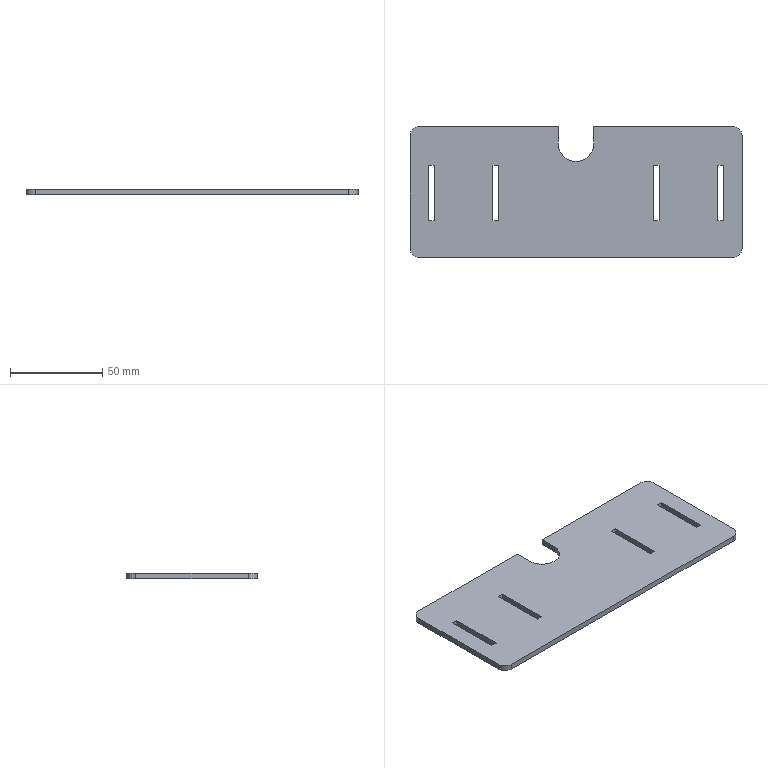Part | SolidWorks | features FlatPattern 1, SMBaseFlange 1, SheetMetal 1 | 1 solid | 30 faces | box 180 x 71 x 3.2 mm | volume 38567 mm3 | plane 25 | cylinder 5 | commonest cylinder face diameters 10 x4 19 x1
STEP:
#1=CARTESIAN_POINT('',(43.2,-230.5,3.2));
#2=VERTEX_POINT('',#1);
#3=CARTESIAN_POINT('',(48.2,-225.5,3.2));
#4=VERTEX_POINT('',#3);
#5=CARTESIAN_POINT('',(43.2,-225.5,3.2));
#6=DIRECTION('',(0.,0.,1.));
#7=DIRECTION('',(1.,0.,0.));
#8=AXIS2_PLACEMENT_3D('',#5,#6,#7);
#9=CIRCLE('',#8,5.);
#10=EDGE_CURVE('',#2,#4,#9,.T.);
#11=ORIENTED_EDGE('',*,*,#10,.T.);
#12=CARTESIAN_POINT('',(48.2,-164.5,3.2));
#13=VERTEX_POINT('',#12);
#14=CARTESIAN_POINT('',(48.2,-164.5,3.2));
#15=DIRECTION('',(0.,1.,0.));
#16=VECTOR('',#15,1000.);
#17=LINE('',#14,#16);
#18=EDGE_CURVE('',#4,#13,#17,.T.);
#19=ORIENTED_EDGE('',*,*,#18,.T.);
#20=CARTESIAN_POINT('',(43.2,-159.5,3.2));
#21=VERTEX_POINT('',#20);
#22=CARTESIAN_POINT('',(43.2,-164.5,3.2));
#23=DIRECTION('',(0.,0.,1.));
#24=DIRECTION('',(1.,0.,0.));
#25=AXIS2_PLACEMENT_3D('',#22,#23,#24);
#26=CIRCLE('',#25,5.);
#27=EDGE_CURVE('',#13,#21,#26,.T.);
#28=ORIENTED_EDGE('',*,*,#27,.T.);
#29=CARTESIAN_POINT('',(-32.3,-159.5,3.2));
#30=VERTEX_POINT('',#29);
#31=CARTESIAN_POINT('',(43.2,-159.5,3.2));
#32=DIRECTION('',(-1.,0.,0.));
#33=VECTOR('',#32,1000.);
#34=LINE('',#31,#33);
#35=EDGE_CURVE('',#21,#30,#34,.T.);
#36=ORIENTED_EDGE('',*,*,#35,.T.);
#37=CARTESIAN_POINT('',(-32.3,-169.,3.2));
#38=VERTEX_POINT('',#37);
#39=CARTESIAN_POINT('',(-32.3,-169.,3.2));
#40=DIRECTION('',(0.,-1.,0.));
#41=VECTOR('',#40,1000.);
#42=LINE('',#39,#41);
#43=EDGE_CURVE('',#30,#38,#42,.T.);
#44=ORIENTED_EDGE('',*,*,#43,.T.);
#45=CARTESIAN_POINT('',(-51.3,-169.,3.2));
#46=VERTEX_POINT('',#45);
#47=CARTESIAN_POINT('',(-41.8,-169.,3.2));
#48=DIRECTION('',(0.,0.,-1.));
#49=DIRECTION('',(1.,0.,0.));
#50=AXIS2_PLACEMENT_3D('',#47,#48,#49);
#51=CIRCLE('',#50,9.5);
#52=EDGE_CURVE('',#38,#46,#51,.T.);
#53=ORIENTED_EDGE('',*,*,#52,.T.);
#54=CARTESIAN_POINT('',(-51.3,-159.5,3.2));
#55=VERTEX_POINT('',#54);
#56=CARTESIAN_POINT('',(-51.3,-169.,3.2));
#57=DIRECTION('',(0.,1.,0.));
#58=VECTOR('',#57,1000.);
#59=LINE('',#56,#58);
#60=EDGE_CURVE('',#46,#55,#59,.T.);
#61=ORIENTED_EDGE('',*,*,#60,.T.);
#62=CARTESIAN_POINT('',(-126.8,-159.5,3.2));
#63=VERTEX_POINT('',#62);
#64=CARTESIAN_POINT('',(-51.3,-159.5,3.2));
#65=DIRECTION('',(-1.,0.,0.));
#66=VECTOR('',#65,1000.);
#67=LINE('',#64,#66);
#68=EDGE_CURVE('',#55,#63,#67,.T.);
#69=ORIENTED_EDGE('',*,*,#68,.T.);
#70=CARTESIAN_POINT('',(-131.8,-164.5,3.2));
#71=VERTEX_POINT('',#70);
#72=CARTESIAN_POINT('',(-126.8,-164.5,3.2));
#73=DIRECTION('',(0.,0.,1.));
#74=DIRECTION('',(-1.,0.,0.));
#75=AXIS2_PLACEMENT_3D('',#72,#73,#74);
#76=CIRCLE('',#75,5.);
#77=EDGE_CURVE('',#63,#71,#76,.T.);
#78=ORIENTED_EDGE('',*,*,#77,.T.);
#79=CARTESIAN_POINT('',(-131.8,-225.5,3.2));
#80=VERTEX_POINT('',#79);
#81=CARTESIAN_POINT('',(-131.8,-164.5,3.2));
#82=DIRECTION('',(0.,-1.,0.));
#83=VECTOR('',#82,1000.);
#84=LINE('',#81,#83);
#85=EDGE_CURVE('',#71,#80,#84,.T.);
#86=ORIENTED_EDGE('',*,*,#85,.T.);
#87=CARTESIAN_POINT('',(-126.8,-230.5,3.2));
#88=VERTEX_POINT('',#87);
#89=CARTESIAN_POINT('',(-126.8,-225.5,3.2));
#90=DIRECTION('',(0.,0.,1.));
#91=DIRECTION('',(-1.,0.,0.));
#92=AXIS2_PLACEMENT_3D('',#89,#90,#91);
#93=CIRCLE('',#92,5.);
#94=EDGE_CURVE('',#80,#88,#93,.T.);
#95=ORIENTED_EDGE('',*,*,#94,.T.);
#96=CARTESIAN_POINT('',(43.2,-230.5,3.2));
#97=DIRECTION('',(1.,0.,0.));
#98=VECTOR('',#97,1000.);
#99=LINE('',#96,#98);
#100=EDGE_CURVE('',#88,#2,#99,.T.);
#101=ORIENTED_EDGE('',*,*,#100,.T.);
#102=EDGE_LOOP('',(#11,#19,#28,#36,#44,#53,#61,#69,#78,#86,#95,#101));
#103=FACE_OUTER_BOUND('',#102,.T.);
#104=CARTESIAN_POINT('',(-121.8,-210.5,3.2));
#105=VERTEX_POINT('',#104);
#106=CARTESIAN_POINT('',(-118.6,-210.5,3.2));
#107=VERTEX_POINT('',#106);
#108=CARTESIAN_POINT('',(-121.8,-210.5,3.2));
#109=DIRECTION('',(1.,0.,0.));
#110=VECTOR('',#109,1000.);
#111=LINE('',#108,#110);
#112=EDGE_CURVE('',#105,#107,#111,.T.);
#113=ORIENTED_EDGE('',*,*,#112,.F.);
#114=CARTESIAN_POINT('',(-121.8,-180.5,3.2));
#115=VERTEX_POINT('',#114);
#116=CARTESIAN_POINT('',(-121.8,-210.5,3.2));
#117=DIRECTION('',(0.,-1.,0.));
#118=VECTOR('',#117,1000.);
#119=LINE('',#116,#118);
#120=EDGE_CURVE('',#115,#105,#119,.T.);
#121=ORIENTED_EDGE('',*,*,#120,.F.);
#122=CARTESIAN_POINT('',(-118.6,-180.5,3.2));
#123=VERTEX_POINT('',#122);
#124=CARTESIAN_POINT('',(-121.8,-180.5,3.2));
#125=DIRECTION('',(-1.,0.,0.));
#126=VECTOR('',#125,1000.);
#127=LINE('',#124,#126);
#128=EDGE_CURVE('',#123,#115,#127,.T.);
#129=ORIENTED_EDGE('',*,*,#128,.F.);
#130=CARTESIAN_POINT('',(-118.6,-210.5,3.2));
#131=DIRECTION('',(0.,1.,0.));
#132=VECTOR('',#131,1000.);
#133=LINE('',#130,#132);
#134=EDGE_CURVE('',#107,#123,#133,.T.);
#135=ORIENTED_EDGE('',*,*,#134,.F.);
#136=EDGE_LOOP('',(#113,#121,#129,#135));
#137=FACE_BOUND('',#136,.T.);
#138=CARTESIAN_POINT('',(-86.8,-210.5,3.2));
#139=VERTEX_POINT('',#138);
#140=CARTESIAN_POINT('',(-83.6,-210.5,3.2));
#141=VERTEX_POINT('',#140);
#142=CARTESIAN_POINT('',(-86.8,-210.5,3.2));
#143=DIRECTION('',(1.,0.,0.));
#144=VECTOR('',#143,1000.);
#145=LINE('',#142,#144);
#146=EDGE_CURVE('',#139,#141,#145,.T.);
#147=ORIENTED_EDGE('',*,*,#146,.F.);
#148=CARTESIAN_POINT('',(-86.8,-180.5,3.2));
#149=VERTEX_POINT('',#148);
#150=CARTESIAN_POINT('',(-86.8,-210.5,3.2));
#151=DIRECTION('',(0.,-1.,0.));
#152=VECTOR('',#151,1000.);
#153=LINE('',#150,#152);
#154=EDGE_CURVE('',#149,#139,#153,.T.);
#155=ORIENTED_EDGE('',*,*,#154,.F.);
#156=CARTESIAN_POINT('',(-83.6,-180.5,3.2));
#157=VERTEX_POINT('',#156);
#158=CARTESIAN_POINT('',(-86.8,-180.5,3.2));
#159=DIRECTION('',(-1.,0.,0.));
#160=VECTOR('',#159,1000.);
#161=LINE('',#158,#160);
#162=EDGE_CURVE('',#157,#149,#161,.T.);
#163=ORIENTED_EDGE('',*,*,#162,.F.);
#164=CARTESIAN_POINT('',(-83.6,-210.5,3.2));
#165=DIRECTION('',(0.,1.,0.));
#166=VECTOR('',#165,1000.);
#167=LINE('',#164,#166);
#168=EDGE_CURVE('',#141,#157,#167,.T.);
#169=ORIENTED_EDGE('',*,*,#168,.F.);
#170=EDGE_LOOP('',(#147,#155,#163,#169));
#171=FACE_BOUND('',#170,.T.);
#172=CARTESIAN_POINT('',(0.,-210.5,3.2));
#173=VERTEX_POINT('',#172);
#174=CARTESIAN_POINT('',(3.2,-210.5,3.2));
#175=VERTEX_POINT('',#174);
#176=CARTESIAN_POINT('',(0.,-210.5,3.2));
#177=DIRECTION('',(1.,0.,0.));
#178=VECTOR('',#177,1000.);
#179=LINE('',#176,#178);
#180=EDGE_CURVE('',#173,#175,#179,.T.);
#181=ORIENTED_EDGE('',*,*,#180,.F.);
#182=CARTESIAN_POINT('',(0.,-180.5,3.2));
#183=VERTEX_POINT('',#182);
#184=CARTESIAN_POINT('',(0.,-210.5,3.2));
#185=DIRECTION('',(0.,-1.,0.));
#186=VECTOR('',#185,1000.);
#187=LINE('',#184,#186);
#188=EDGE_CURVE('',#183,#173,#187,.T.);
#189=ORIENTED_EDGE('',*,*,#188,.F.);
#190=CARTESIAN_POINT('',(3.2,-180.5,3.2));
#191=VERTEX_POINT('',#190);
#192=CARTESIAN_POINT('',(0.,-180.5,3.2));
#193=DIRECTION('',(-1.,0.,0.));
#194=VECTOR('',#193,1000.);
#195=LINE('',#192,#194);
#196=EDGE_CURVE('',#191,#183,#195,.T.);
#197=ORIENTED_EDGE('',*,*,#196,.F.);
#198=CARTESIAN_POINT('',(3.2,-210.5,3.2));
#199=DIRECTION('',(0.,1.,0.));
#200=VECTOR('',#199,1000.);
#201=LINE('',#198,#200);
#202=EDGE_CURVE('',#175,#191,#201,.T.);
#203=ORIENTED_EDGE('',*,*,#202,.F.);
#204=EDGE_LOOP('',(#181,#189,#197,#203));
#205=FACE_BOUND('',#204,.T.);
#206=CARTESIAN_POINT('',(35.,-210.5,3.2));
#207=VERTEX_POINT('',#206);
#208=CARTESIAN_POINT('',(38.2,-210.5,3.2));
#209=VERTEX_POINT('',#208);
#210=CARTESIAN_POINT('',(35.,-210.5,3.2));
#211=DIRECTION('',(1.,0.,0.));
#212=VECTOR('',#211,1000.);
#213=LINE('',#210,#212);
#214=EDGE_CURVE('',#207,#209,#213,.T.);
#215=ORIENTED_EDGE('',*,*,#214,.F.);
#216=CARTESIAN_POINT('',(35.,-180.5,3.2));
#217=VERTEX_POINT('',#216);
#218=CARTESIAN_POINT('',(35.,-210.5,3.2));
#219=DIRECTION('',(0.,-1.,0.));
#220=VECTOR('',#219,1000.);
#221=LINE('',#218,#220);
#222=EDGE_CURVE('',#217,#207,#221,.T.);
#223=ORIENTED_EDGE('',*,*,#222,.F.);
#224=CARTESIAN_POINT('',(38.2,-180.5,3.2));
#225=VERTEX_POINT('',#224);
#226=CARTESIAN_POINT('',(35.,-180.5,3.2));
#227=DIRECTION('',(-1.,0.,0.));
#228=VECTOR('',#227,1000.);
#229=LINE('',#226,#228);
#230=EDGE_CURVE('',#225,#217,#229,.T.);
#231=ORIENTED_EDGE('',*,*,#230,.F.);
#232=CARTESIAN_POINT('',(38.2,-210.5,3.2));
#233=DIRECTION('',(0.,1.,0.));
#234=VECTOR('',#233,1000.);
#235=LINE('',#232,#234);
#236=EDGE_CURVE('',#209,#225,#235,.T.);
#237=ORIENTED_EDGE('',*,*,#236,.F.);
#238=EDGE_LOOP('',(#215,#223,#231,#237));
#239=FACE_BOUND('',#238,.T.);
#240=CARTESIAN_POINT('',(43.2,-225.5,3.2));
#241=DIRECTION('',(0.,0.,1.));
#242=DIRECTION('',(1.,0.,0.));
#243=AXIS2_PLACEMENT_3D('',#240,#241,#242);
#244=PLANE('',#243);
#245=ADVANCED_FACE('',(#103,#137,#171,#205,#239),#244,.T.);
#246=CARTESIAN_POINT('',(0.,-180.5,0.));
#247=VERTEX_POINT('',#246);
#248=CARTESIAN_POINT('',(0.,-210.5,0.));
#249=VERTEX_POINT('',#248);
#250=CARTESIAN_POINT('',(0.,-210.5,0.));
#251=DIRECTION('',(0.,-1.,0.));
#252=VECTOR('',#251,1000.);
#253=LINE('',#250,#252);
#254=EDGE_CURVE('',#247,#249,#253,.T.);
#255=ORIENTED_EDGE('',*,*,#254,.T.);
#256=CARTESIAN_POINT('',(3.2,-210.5,0.));
#257=VERTEX_POINT('',#256);
#258=CARTESIAN_POINT('',(0.,-210.5,0.));
#259=DIRECTION('',(1.,0.,0.));
#260=VECTOR('',#259,1000.);
#261=LINE('',#258,#260);
#262=EDGE_CURVE('',#249,#257,#261,.T.);
#263=ORIENTED_EDGE('',*,*,#262,.T.);
#264=CARTESIAN_POINT('',(3.2,-180.5,0.));
#265=VERTEX_POINT('',#264);
#266=CARTESIAN_POINT('',(3.2,-210.5,0.));
#267=DIRECTION('',(0.,1.,0.));
#268=VECTOR('',#267,1000.);
#269=LINE('',#266,#268);
#270=EDGE_CURVE('',#257,#265,#269,.T.);
#271=ORIENTED_EDGE('',*,*,#270,.T.);
#272=CARTESIAN_POINT('',(0.,-180.5,0.));
#273=DIRECTION('',(-1.,0.,0.));
#274=VECTOR('',#273,1000.);
#275=LINE('',#272,#274);
#276=EDGE_CURVE('',#265,#247,#275,.T.);
#277=ORIENTED_EDGE('',*,*,#276,.T.);
#278=EDGE_LOOP('',(#255,#263,#271,#277));
#279=FACE_BOUND('',#278,.T.);
#280=CARTESIAN_POINT('',(-121.8,-180.5,0.));
#281=VERTEX_POINT('',#280);
#282=CARTESIAN_POINT('',(-121.8,-210.5,0.));
#283=VERTEX_POINT('',#282);
#284=CARTESIAN_POINT('',(-121.8,-210.5,0.));
#285=DIRECTION('',(0.,-1.,0.));
#286=VECTOR('',#285,1000.);
#287=LINE('',#284,#286);
#288=EDGE_CURVE('',#281,#283,#287,.T.);
#289=ORIENTED_EDGE('',*,*,#288,.T.);
#290=CARTESIAN_POINT('',(-118.6,-210.5,0.));
#291=VERTEX_POINT('',#290);
#292=CARTESIAN_POINT('',(-121.8,-210.5,0.));
#293=DIRECTION('',(1.,0.,0.));
#294=VECTOR('',#293,1000.);
#295=LINE('',#292,#294);
#296=EDGE_CURVE('',#283,#291,#295,.T.);
#297=ORIENTED_EDGE('',*,*,#296,.T.);
#298=CARTESIAN_POINT('',(-118.6,-180.5,0.));
#299=VERTEX_POINT('',#298);
#300=CARTESIAN_POINT('',(-118.6,-210.5,0.));
#301=DIRECTION('',(0.,1.,0.));
#302=VECTOR('',#301,1000.);
#303=LINE('',#300,#302);
#304=EDGE_CURVE('',#291,#299,#303,.T.);
#305=ORIENTED_EDGE('',*,*,#304,.T.);
#306=CARTESIAN_POINT('',(-121.8,-180.5,0.));
#307=DIRECTION('',(-1.,0.,0.));
#308=VECTOR('',#307,1000.);
#309=LINE('',#306,#308);
#310=EDGE_CURVE('',#299,#281,#309,.T.);
#311=ORIENTED_EDGE('',*,*,#310,.T.);
#312=EDGE_LOOP('',(#289,#297,#305,#311));
#313=FACE_BOUND('',#312,.T.);
#314=CARTESIAN_POINT('',(43.2,-230.5,0.));
#315=VERTEX_POINT('',#314);
#316=CARTESIAN_POINT('',(48.2,-225.5,0.));
#317=VERTEX_POINT('',#316);
#318=CARTESIAN_POINT('',(43.2,-225.5,0.));
#319=DIRECTION('',(0.,0.,1.));
#320=DIRECTION('',(1.,0.,0.));
#321=AXIS2_PLACEMENT_3D('',#318,#319,#320);
#322=CIRCLE('',#321,5.);
#323=EDGE_CURVE('',#315,#317,#322,.T.);
#324=ORIENTED_EDGE('',*,*,#323,.F.);
#325=CARTESIAN_POINT('',(-126.8,-230.5,0.));
#326=VERTEX_POINT('',#325);
#327=CARTESIAN_POINT('',(43.2,-230.5,0.));
#328=DIRECTION('',(1.,0.,0.));
#329=VECTOR('',#328,1000.);
#330=LINE('',#327,#329);
#331=EDGE_CURVE('',#326,#315,#330,.T.);
#332=ORIENTED_EDGE('',*,*,#331,.F.);
#333=CARTESIAN_POINT('',(-131.8,-225.5,0.));
#334=VERTEX_POINT('',#333);
#335=CARTESIAN_POINT('',(-126.8,-225.5,0.));
#336=DIRECTION('',(0.,0.,1.));
#337=DIRECTION('',(-1.,0.,0.));
#338=AXIS2_PLACEMENT_3D('',#335,#336,#337);
#339=CIRCLE('',#338,5.);
#340=EDGE_CURVE('',#334,#326,#339,.T.);
#341=ORIENTED_EDGE('',*,*,#340,.F.);
#342=CARTESIAN_POINT('',(-131.8,-164.5,0.));
#343=VERTEX_POINT('',#342);
#344=CARTESIAN_POINT('',(-131.8,-164.5,0.));
#345=DIRECTION('',(0.,-1.,0.));
#346=VECTOR('',#345,1000.);
#347=LINE('',#344,#346);
#348=EDGE_CURVE('',#343,#334,#347,.T.);
#349=ORIENTED_EDGE('',*,*,#348,.F.);
#350=CARTESIAN_POINT('',(-126.8,-159.5,0.));
#351=VERTEX_POINT('',#350);
#352=CARTESIAN_POINT('',(-126.8,-164.5,0.));
#353=DIRECTION('',(0.,0.,1.));
#354=DIRECTION('',(-1.,0.,0.));
#355=AXIS2_PLACEMENT_3D('',#352,#353,#354);
#356=CIRCLE('',#355,5.);
#357=EDGE_CURVE('',#351,#343,#356,.T.);
#358=ORIENTED_EDGE('',*,*,#357,.F.);
#359=CARTESIAN_POINT('',(-51.3,-159.5,0.));
#360=VERTEX_POINT('',#359);
#361=CARTESIAN_POINT('',(-51.3,-159.5,0.));
#362=DIRECTION('',(-1.,0.,0.));
#363=VECTOR('',#362,1000.);
#364=LINE('',#361,#363);
#365=EDGE_CURVE('',#360,#351,#364,.T.);
#366=ORIENTED_EDGE('',*,*,#365,.F.);
#367=CARTESIAN_POINT('',(-51.3,-169.,0.));
#368=VERTEX_POINT('',#367);
#369=CARTESIAN_POINT('',(-51.3,-169.,0.));
#370=DIRECTION('',(0.,1.,0.));
#371=VECTOR('',#370,1000.);
#372=LINE('',#369,#371);
#373=EDGE_CURVE('',#368,#360,#372,.T.);
#374=ORIENTED_EDGE('',*,*,#373,.F.);
#375=CARTESIAN_POINT('',(-32.3,-169.,0.));
#376=VERTEX_POINT('',#375);
#377=CARTESIAN_POINT('',(-41.8,-169.,0.));
#378=DIRECTION('',(0.,0.,-1.));
#379=DIRECTION('',(1.,0.,0.));
#380=AXIS2_PLACEMENT_3D('',#377,#378,#379);
#381=CIRCLE('',#380,9.5);
#382=EDGE_CURVE('',#376,#368,#381,.T.);
#383=ORIENTED_EDGE('',*,*,#382,.F.);
#384=CARTESIAN_POINT('',(-32.3,-159.5,0.));
#385=VERTEX_POINT('',#384);
#386=CARTESIAN_POINT('',(-32.3,-169.,0.));
#387=DIRECTION('',(0.,-1.,0.));
#388=VECTOR('',#387,1000.);
#389=LINE('',#386,#388);
#390=EDGE_CURVE('',#385,#376,#389,.T.);
#391=ORIENTED_EDGE('',*,*,#390,.F.);
#392=CARTESIAN_POINT('',(43.2,-159.5,0.));
#393=VERTEX_POINT('',#392);
#394=CARTESIAN_POINT('',(43.2,-159.5,0.));
#395=DIRECTION('',(-1.,0.,0.));
#396=VECTOR('',#395,1000.);
#397=LINE('',#394,#396);
#398=EDGE_CURVE('',#393,#385,#397,.T.);
#399=ORIENTED_EDGE('',*,*,#398,.F.);
#400=CARTESIAN_POINT('',(48.2,-164.5,0.));
#401=VERTEX_POINT('',#400);
#402=CARTESIAN_POINT('',(43.2,-164.5,0.));
#403=DIRECTION('',(0.,0.,1.));
#404=DIRECTION('',(1.,0.,0.));
#405=AXIS2_PLACEMENT_3D('',#402,#403,#404);
#406=CIRCLE('',#405,5.);
#407=EDGE_CURVE('',#401,#393,#406,.T.);
#408=ORIENTED_EDGE('',*,*,#407,.F.);
#409=CARTESIAN_POINT('',(48.2,-164.5,0.));
#410=DIRECTION('',(0.,1.,0.));
#411=VECTOR('',#410,1000.);
#412=LINE('',#409,#411);
#413=EDGE_CURVE('',#317,#401,#412,.T.);
#414=ORIENTED_EDGE('',*,*,#413,.F.);
#415=EDGE_LOOP('',(#324,#332,#341,#349,#358,#366,#374,#383,#391,#399,#408,#414));
#416=FACE_OUTER_BOUND('',#415,.T.);
#417=CARTESIAN_POINT('',(-86.8,-180.5,0.));
#418=VERTEX_POINT('',#417);
#419=CARTESIAN_POINT('',(-86.8,-210.5,0.));
#420=VERTEX_POINT('',#419);
#421=CARTESIAN_POINT('',(-86.8,-210.5,0.));
#422=DIRECTION('',(0.,-1.,0.));
#423=VECTOR('',#422,1000.);
#424=LINE('',#421,#423);
#425=EDGE_CURVE('',#418,#420,#424,.T.);
#426=ORIENTED_EDGE('',*,*,#425,.T.);
#427=CARTESIAN_POINT('',(-83.6,-210.5,0.));
#428=VERTEX_POINT('',#427);
#429=CARTESIAN_POINT('',(-86.8,-210.5,0.));
#430=DIRECTION('',(1.,0.,0.));
#431=VECTOR('',#430,1000.);
#432=LINE('',#429,#431);
#433=EDGE_CURVE('',#420,#428,#432,.T.);
#434=ORIENTED_EDGE('',*,*,#433,.T.);
#435=CARTESIAN_POINT('',(-83.6,-180.5,0.));
#436=VERTEX_POINT('',#435);
#437=CARTESIAN_POINT('',(-83.6,-210.5,0.));
#438=DIRECTION('',(0.,1.,0.));
#439=VECTOR('',#438,1000.);
#440=LINE('',#437,#439);
#441=EDGE_CURVE('',#428,#436,#440,.T.);
#442=ORIENTED_EDGE('',*,*,#441,.T.);
#443=CARTESIAN_POINT('',(-86.8,-180.5,0.));
#444=DIRECTION('',(-1.,0.,0.));
#445=VECTOR('',#444,1000.);
#446=LINE('',#443,#445);
#447=EDGE_CURVE('',#436,#418,#446,.T.);
#448=ORIENTED_EDGE('',*,*,#447,.T.);
#449=EDGE_LOOP('',(#426,#434,#442,#448));
#450=FACE_BOUND('',#449,.T.);
#451=CARTESIAN_POINT('',(35.,-180.5,0.));
#452=VERTEX_POINT('',#451);
#453=CARTESIAN_POINT('',(35.,-210.5,0.));
#454=VERTEX_POINT('',#453);
#455=CARTESIAN_POINT('',(35.,-210.5,0.));
#456=DIRECTION('',(0.,-1.,0.));
#457=VECTOR('',#456,1000.);
#458=LINE('',#455,#457);
#459=EDGE_CURVE('',#452,#454,#458,.T.);
#460=ORIENTED_EDGE('',*,*,#459,.T.);
#461=CARTESIAN_POINT('',(38.2,-210.5,0.));
#462=VERTEX_POINT('',#461);
#463=CARTESIAN_POINT('',(35.,-210.5,0.));
#464=DIRECTION('',(1.,0.,0.));
#465=VECTOR('',#464,1000.);
#466=LINE('',#463,#465);
#467=EDGE_CURVE('',#454,#462,#466,.T.);
#468=ORIENTED_EDGE('',*,*,#467,.T.);
#469=CARTESIAN_POINT('',(38.2,-180.5,0.));
#470=VERTEX_POINT('',#469);
#471=CARTESIAN_POINT('',(38.2,-210.5,0.));
#472=DIRECTION('',(0.,1.,0.));
#473=VECTOR('',#472,1000.);
#474=LINE('',#471,#473);
#475=EDGE_CURVE('',#462,#470,#474,.T.);
#476=ORIENTED_EDGE('',*,*,#475,.T.);
#477=CARTESIAN_POINT('',(35.,-180.5,0.));
#478=DIRECTION('',(-1.,0.,0.));
#479=VECTOR('',#478,1000.);
#480=LINE('',#477,#479);
#481=EDGE_CURVE('',#470,#452,#480,.T.);
#482=ORIENTED_EDGE('',*,*,#481,.T.);
#483=EDGE_LOOP('',(#460,#468,#476,#482));
#484=FACE_BOUND('',#483,.T.);
#485=CARTESIAN_POINT('',(43.2,-225.5,0.));
#486=DIRECTION('',(0.,0.,1.));
#487=DIRECTION('',(1.,0.,0.));
#488=AXIS2_PLACEMENT_3D('',#485,#486,#487);
#489=PLANE('',#488);
#490=ADVANCED_FACE('',(#279,#313,#416,#450,#484),#489,.F.);
#491=ORIENTED_EDGE('',*,*,#323,.T.);
#492=CARTESIAN_POINT('',(48.2,-225.5,3.2));
#493=DIRECTION('',(0.,0.,-1.));
#494=VECTOR('',#493,1000.);
#495=LINE('',#492,#494);
#496=EDGE_CURVE('',#4,#317,#495,.T.);
#497=ORIENTED_EDGE('',*,*,#496,.F.);
#498=ORIENTED_EDGE('',*,*,#10,.F.);
#499=CARTESIAN_POINT('',(43.2,-230.5,3.2));
#500=DIRECTION('',(0.,0.,-1.));
#501=VECTOR('',#500,1000.);
#502=LINE('',#499,#501);
#503=EDGE_CURVE('',#2,#315,#502,.T.);
#504=ORIENTED_EDGE('',*,*,#503,.T.);
#505=EDGE_LOOP('',(#491,#497,#498,#504));
#506=FACE_OUTER_BOUND('',#505,.T.);
#507=CARTESIAN_POINT('',(43.2,-225.5,3.2));
#508=DIRECTION('',(0.,0.,-1.));
#509=DIRECTION('',(-1.,0.,0.));
#510=AXIS2_PLACEMENT_3D('',#507,#508,#509);
#511=CYLINDRICAL_SURFACE('',#510,5.);
#512=ADVANCED_FACE('',(#506),#511,.T.);
#513=ORIENTED_EDGE('',*,*,#413,.T.);
#514=CARTESIAN_POINT('',(48.2,-164.5,3.2));
#515=DIRECTION('',(0.,0.,-1.));
#516=VECTOR('',#515,1000.);
#517=LINE('',#514,#516);
#518=EDGE_CURVE('',#13,#401,#517,.T.);
#519=ORIENTED_EDGE('',*,*,#518,.F.);
#520=ORIENTED_EDGE('',*,*,#18,.F.);
#521=ORIENTED_EDGE('',*,*,#496,.T.);
#522=EDGE_LOOP('',(#513,#519,#520,#521));
#523=FACE_OUTER_BOUND('',#522,.T.);
#524=CARTESIAN_POINT('',(48.2,-164.5,3.2));
#525=DIRECTION('',(-1.,0.,0.));
#526=DIRECTION('',(0.,-1.,0.));
#527=AXIS2_PLACEMENT_3D('',#524,#525,#526);
#528=PLANE('',#527);
#529=ADVANCED_FACE('',(#523),#528,.F.);
#530=ORIENTED_EDGE('',*,*,#407,.T.);
#531=CARTESIAN_POINT('',(43.2,-159.5,3.2));
#532=DIRECTION('',(0.,0.,-1.));
#533=VECTOR('',#532,1000.);
#534=LINE('',#531,#533);
#535=EDGE_CURVE('',#21,#393,#534,.T.);
#536=ORIENTED_EDGE('',*,*,#535,.F.);
#537=ORIENTED_EDGE('',*,*,#27,.F.);
#538=ORIENTED_EDGE('',*,*,#518,.T.);
#539=EDGE_LOOP('',(#530,#536,#537,#538));
#540=FACE_OUTER_BOUND('',#539,.T.);
#541=CARTESIAN_POINT('',(43.2,-164.5,3.2));
#542=DIRECTION('',(0.,0.,-1.));
#543=DIRECTION('',(-1.,0.,0.));
#544=AXIS2_PLACEMENT_3D('',#541,#542,#543);
#545=CYLINDRICAL_SURFACE('',#544,5.);
#546=ADVANCED_FACE('',(#540),#545,.T.);
#547=ORIENTED_EDGE('',*,*,#398,.T.);
#548=CARTESIAN_POINT('',(-32.3,-159.5,3.2));
#549=DIRECTION('',(0.,0.,-1.));
#550=VECTOR('',#549,1000.);
#551=LINE('',#548,#550);
#552=EDGE_CURVE('',#30,#385,#551,.T.);
#553=ORIENTED_EDGE('',*,*,#552,.F.);
#554=ORIENTED_EDGE('',*,*,#35,.F.);
#555=ORIENTED_EDGE('',*,*,#535,.T.);
#556=EDGE_LOOP('',(#547,#553,#554,#555));
#557=FACE_OUTER_BOUND('',#556,.T.);
#558=CARTESIAN_POINT('',(43.2,-159.5,3.2));
#559=DIRECTION('',(0.,-1.,0.));
#560=DIRECTION('',(0.,0.,-1.));
#561=AXIS2_PLACEMENT_3D('',#558,#559,#560);
#562=PLANE('',#561);
#563=ADVANCED_FACE('',(#557),#562,.F.);
#564=ORIENTED_EDGE('',*,*,#390,.T.);
#565=CARTESIAN_POINT('',(-32.3,-169.,3.2));
#566=DIRECTION('',(0.,0.,-1.));
#567=VECTOR('',#566,1000.);
#568=LINE('',#565,#567);
#569=EDGE_CURVE('',#38,#376,#568,.T.);
#570=ORIENTED_EDGE('',*,*,#569,.F.);
#571=ORIENTED_EDGE('',*,*,#43,.F.);
#572=ORIENTED_EDGE('',*,*,#552,.T.);
#573=EDGE_LOOP('',(#564,#570,#571,#572));
#574=FACE_OUTER_BOUND('',#573,.T.);
#575=CARTESIAN_POINT('',(-32.3,-169.,3.2));
#576=DIRECTION('',(1.,0.,0.));
#577=DIRECTION('',(0.,1.,0.));
#578=AXIS2_PLACEMENT_3D('',#575,#576,#577);
#579=PLANE('',#578);
#580=ADVANCED_FACE('',(#574),#579,.F.);
#581=ORIENTED_EDGE('',*,*,#382,.T.);
#582=CARTESIAN_POINT('',(-51.3,-169.,3.2));
#583=DIRECTION('',(0.,0.,-1.));
#584=VECTOR('',#583,1000.);
#585=LINE('',#582,#584);
#586=EDGE_CURVE('',#46,#368,#585,.T.);
#587=ORIENTED_EDGE('',*,*,#586,.F.);
#588=ORIENTED_EDGE('',*,*,#52,.F.);
#589=ORIENTED_EDGE('',*,*,#569,.T.);
#590=EDGE_LOOP('',(#581,#587,#588,#589));
#591=FACE_OUTER_BOUND('',#590,.T.);
#592=CARTESIAN_POINT('',(-41.8,-169.,3.2));
#593=DIRECTION('',(0.,0.,-1.));
#594=DIRECTION('',(-1.,0.,0.));
#595=AXIS2_PLACEMENT_3D('',#592,#593,#594);
#596=CYLINDRICAL_SURFACE('',#595,9.5);
#597=ADVANCED_FACE('',(#591),#596,.F.);
#598=ORIENTED_EDGE('',*,*,#373,.T.);
#599=CARTESIAN_POINT('',(-51.3,-159.5,3.2));
#600=DIRECTION('',(0.,0.,-1.));
#601=VECTOR('',#600,1000.);
#602=LINE('',#599,#601);
#603=EDGE_CURVE('',#55,#360,#602,.T.);
#604=ORIENTED_EDGE('',*,*,#603,.F.);
#605=ORIENTED_EDGE('',*,*,#60,.F.);
#606=ORIENTED_EDGE('',*,*,#586,.T.);
#607=EDGE_LOOP('',(#598,#604,#605,#606));
#608=FACE_OUTER_BOUND('',#607,.T.);
#609=CARTESIAN_POINT('',(-51.3,-169.,3.2));
#610=DIRECTION('',(-1.,0.,0.));
#611=DIRECTION('',(0.,-1.,0.));
#612=AXIS2_PLACEMENT_3D('',#609,#610,#611);
#613=PLANE('',#612);
#614=ADVANCED_FACE('',(#608),#613,.F.);
#615=ORIENTED_EDGE('',*,*,#365,.T.);
#616=CARTESIAN_POINT('',(-126.8,-159.5,3.2));
#617=DIRECTION('',(0.,0.,-1.));
#618=VECTOR('',#617,1000.);
#619=LINE('',#616,#618);
#620=EDGE_CURVE('',#63,#351,#619,.T.);
#621=ORIENTED_EDGE('',*,*,#620,.F.);
#622=ORIENTED_EDGE('',*,*,#68,.F.);
#623=ORIENTED_EDGE('',*,*,#603,.T.);
#624=EDGE_LOOP('',(#615,#621,#622,#623));
#625=FACE_OUTER_BOUND('',#624,.T.);
#626=CARTESIAN_POINT('',(-51.3,-159.5,3.2));
#627=DIRECTION('',(0.,-1.,0.));
#628=DIRECTION('',(0.,0.,-1.));
#629=AXIS2_PLACEMENT_3D('',#626,#627,#628);
#630=PLANE('',#629);
#631=ADVANCED_FACE('',(#625),#630,.F.);
#632=ORIENTED_EDGE('',*,*,#357,.T.);
#633=CARTESIAN_POINT('',(-131.8,-164.5,3.2));
#634=DIRECTION('',(0.,0.,-1.));
#635=VECTOR('',#634,1000.);
#636=LINE('',#633,#635);
#637=EDGE_CURVE('',#71,#343,#636,.T.);
#638=ORIENTED_EDGE('',*,*,#637,.F.);
#639=ORIENTED_EDGE('',*,*,#77,.F.);
#640=ORIENTED_EDGE('',*,*,#620,.T.);
#641=EDGE_LOOP('',(#632,#638,#639,#640));
#642=FACE_OUTER_BOUND('',#641,.T.);
#643=CARTESIAN_POINT('',(-126.8,-164.5,3.2));
#644=DIRECTION('',(0.,0.,-1.));
#645=DIRECTION('',(-1.,0.,0.));
#646=AXIS2_PLACEMENT_3D('',#643,#644,#645);
#647=CYLINDRICAL_SURFACE('',#646,5.);
#648=ADVANCED_FACE('',(#642),#647,.T.);
#649=ORIENTED_EDGE('',*,*,#348,.T.);
#650=CARTESIAN_POINT('',(-131.8,-225.5,3.2));
#651=DIRECTION('',(0.,0.,-1.));
#652=VECTOR('',#651,1000.);
#653=LINE('',#650,#652);
#654=EDGE_CURVE('',#80,#334,#653,.T.);
#655=ORIENTED_EDGE('',*,*,#654,.F.);
#656=ORIENTED_EDGE('',*,*,#85,.F.);
#657=ORIENTED_EDGE('',*,*,#637,.T.);
#658=EDGE_LOOP('',(#649,#655,#656,#657));
#659=FACE_OUTER_BOUND('',#658,.T.);
#660=CARTESIAN_POINT('',(-131.8,-164.5,3.2));
#661=DIRECTION('',(1.,0.,0.));
#662=DIRECTION('',(0.,1.,0.));
#663=AXIS2_PLACEMENT_3D('',#660,#661,#662);
#664=PLANE('',#663);
#665=ADVANCED_FACE('',(#659),#664,.F.);
#666=ORIENTED_EDGE('',*,*,#340,.T.);
#667=CARTESIAN_POINT('',(-126.8,-230.5,3.2));
#668=DIRECTION('',(0.,0.,-1.));
#669=VECTOR('',#668,1000.);
#670=LINE('',#667,#669);
#671=EDGE_CURVE('',#88,#326,#670,.T.);
#672=ORIENTED_EDGE('',*,*,#671,.F.);
#673=ORIENTED_EDGE('',*,*,#94,.F.);
#674=ORIENTED_EDGE('',*,*,#654,.T.);
#675=EDGE_LOOP('',(#666,#672,#673,#674));
#676=FACE_OUTER_BOUND('',#675,.T.);
#677=CARTESIAN_POINT('',(-126.8,-225.5,3.2));
#678=DIRECTION('',(0.,0.,-1.));
#679=DIRECTION('',(-1.,0.,0.));
#680=AXIS2_PLACEMENT_3D('',#677,#678,#679);
#681=CYLINDRICAL_SURFACE('',#680,5.);
#682=ADVANCED_FACE('',(#676),#681,.T.);
#683=ORIENTED_EDGE('',*,*,#331,.T.);
#684=ORIENTED_EDGE('',*,*,#503,.F.);
#685=ORIENTED_EDGE('',*,*,#100,.F.);
#686=ORIENTED_EDGE('',*,*,#671,.T.);
#687=EDGE_LOOP('',(#683,#684,#685,#686));
#688=FACE_OUTER_BOUND('',#687,.T.);
#689=CARTESIAN_POINT('',(43.2,-230.5,3.2));
#690=DIRECTION('',(0.,1.,0.));
#691=DIRECTION('',(0.,0.,1.));
#692=AXIS2_PLACEMENT_3D('',#689,#690,#691);
#693=PLANE('',#692);
#694=ADVANCED_FACE('',(#688),#693,.F.);
#695=ORIENTED_EDGE('',*,*,#288,.F.);
#696=CARTESIAN_POINT('',(-121.8,-180.5,3.2));
#697=DIRECTION('',(0.,0.,-1.));
#698=VECTOR('',#697,1000.);
#699=LINE('',#696,#698);
#700=EDGE_CURVE('',#115,#281,#699,.T.);
#701=ORIENTED_EDGE('',*,*,#700,.F.);
#702=ORIENTED_EDGE('',*,*,#120,.T.);
#703=CARTESIAN_POINT('',(-121.8,-210.5,3.2));
#704=DIRECTION('',(0.,0.,-1.));
#705=VECTOR('',#704,1000.);
#706=LINE('',#703,#705);
#707=EDGE_CURVE('',#105,#283,#706,.T.);
#708=ORIENTED_EDGE('',*,*,#707,.T.);
#709=EDGE_LOOP('',(#695,#701,#702,#708));
#710=FACE_OUTER_BOUND('',#709,.T.);
#711=CARTESIAN_POINT('',(-121.8,-210.5,3.2));
#712=DIRECTION('',(1.,0.,0.));
#713=DIRECTION('',(0.,0.,-1.));
#714=AXIS2_PLACEMENT_3D('',#711,#712,#713);
#715=PLANE('',#714);
#716=ADVANCED_FACE('',(#710),#715,.T.);
#717=ORIENTED_EDGE('',*,*,#296,.F.);
#718=ORIENTED_EDGE('',*,*,#707,.F.);
#719=ORIENTED_EDGE('',*,*,#112,.T.);
#720=CARTESIAN_POINT('',(-118.6,-210.5,3.2));
#721=DIRECTION('',(0.,0.,-1.));
#722=VECTOR('',#721,1000.);
#723=LINE('',#720,#722);
#724=EDGE_CURVE('',#107,#291,#723,.T.);
#725=ORIENTED_EDGE('',*,*,#724,.T.);
#726=EDGE_LOOP('',(#717,#718,#719,#725));
#727=FACE_OUTER_BOUND('',#726,.T.);
#728=CARTESIAN_POINT('',(-121.8,-210.5,3.2));
#729=DIRECTION('',(0.,1.,0.));
#730=DIRECTION('',(0.,0.,1.));
#731=AXIS2_PLACEMENT_3D('',#728,#729,#730);
#732=PLANE('',#731);
#733=ADVANCED_FACE('',(#727),#732,.T.);
#734=ORIENTED_EDGE('',*,*,#304,.F.);
#735=ORIENTED_EDGE('',*,*,#724,.F.);
#736=ORIENTED_EDGE('',*,*,#134,.T.);
#737=CARTESIAN_POINT('',(-118.6,-180.5,3.2));
#738=DIRECTION('',(0.,0.,-1.));
#739=VECTOR('',#738,1000.);
#740=LINE('',#737,#739);
#741=EDGE_CURVE('',#123,#299,#740,.T.);
#742=ORIENTED_EDGE('',*,*,#741,.T.);
#743=EDGE_LOOP('',(#734,#735,#736,#742));
#744=FACE_OUTER_BOUND('',#743,.T.);
#745=CARTESIAN_POINT('',(-118.6,-210.5,3.2));
#746=DIRECTION('',(-1.,0.,0.));
#747=DIRECTION('',(0.,0.,1.));
#748=AXIS2_PLACEMENT_3D('',#745,#746,#747);
#749=PLANE('',#748);
#750=ADVANCED_FACE('',(#744),#749,.T.);
#751=ORIENTED_EDGE('',*,*,#310,.F.);
#752=ORIENTED_EDGE('',*,*,#741,.F.);
#753=ORIENTED_EDGE('',*,*,#128,.T.);
#754=ORIENTED_EDGE('',*,*,#700,.T.);
#755=EDGE_LOOP('',(#751,#752,#753,#754));
#756=FACE_OUTER_BOUND('',#755,.T.);
#757=CARTESIAN_POINT('',(-121.8,-180.5,3.2));
#758=DIRECTION('',(0.,-1.,0.));
#759=DIRECTION('',(0.,0.,-1.));
#760=AXIS2_PLACEMENT_3D('',#757,#758,#759);
#761=PLANE('',#760);
#762=ADVANCED_FACE('',(#756),#761,.T.);
#763=ORIENTED_EDGE('',*,*,#425,.F.);
#764=CARTESIAN_POINT('',(-86.8,-180.5,3.2));
#765=DIRECTION('',(0.,0.,-1.));
#766=VECTOR('',#765,1000.);
#767=LINE('',#764,#766);
#768=EDGE_CURVE('',#149,#418,#767,.T.);
#769=ORIENTED_EDGE('',*,*,#768,.F.);
#770=ORIENTED_EDGE('',*,*,#154,.T.);
#771=CARTESIAN_POINT('',(-86.8,-210.5,3.2));
#772=DIRECTION('',(0.,0.,-1.));
#773=VECTOR('',#772,1000.);
#774=LINE('',#771,#773);
#775=EDGE_CURVE('',#139,#420,#774,.T.);
#776=ORIENTED_EDGE('',*,*,#775,.T.);
#777=EDGE_LOOP('',(#763,#769,#770,#776));
#778=FACE_OUTER_BOUND('',#777,.T.);
#779=CARTESIAN_POINT('',(-86.8,-210.5,3.2));
#780=DIRECTION('',(1.,0.,0.));
#781=DIRECTION('',(0.,0.,-1.));
#782=AXIS2_PLACEMENT_3D('',#779,#780,#781);
#783=PLANE('',#782);
#784=ADVANCED_FACE('',(#778),#783,.T.);
#785=ORIENTED_EDGE('',*,*,#433,.F.);
#786=ORIENTED_EDGE('',*,*,#775,.F.);
#787=ORIENTED_EDGE('',*,*,#146,.T.);
#788=CARTESIAN_POINT('',(-83.6,-210.5,3.2));
#789=DIRECTION('',(0.,0.,-1.));
#790=VECTOR('',#789,1000.);
#791=LINE('',#788,#790);
#792=EDGE_CURVE('',#141,#428,#791,.T.);
#793=ORIENTED_EDGE('',*,*,#792,.T.);
#794=EDGE_LOOP('',(#785,#786,#787,#793));
#795=FACE_OUTER_BOUND('',#794,.T.);
#796=CARTESIAN_POINT('',(-86.8,-210.5,3.2));
#797=DIRECTION('',(0.,1.,0.));
#798=DIRECTION('',(0.,0.,1.));
#799=AXIS2_PLACEMENT_3D('',#796,#797,#798);
#800=PLANE('',#799);
#801=ADVANCED_FACE('',(#795),#800,.T.);
#802=ORIENTED_EDGE('',*,*,#441,.F.);
#803=ORIENTED_EDGE('',*,*,#792,.F.);
#804=ORIENTED_EDGE('',*,*,#168,.T.);
#805=CARTESIAN_POINT('',(-83.6,-180.5,3.2));
#806=DIRECTION('',(0.,0.,-1.));
#807=VECTOR('',#806,1000.);
#808=LINE('',#805,#807);
#809=EDGE_CURVE('',#157,#436,#808,.T.);
#810=ORIENTED_EDGE('',*,*,#809,.T.);
#811=EDGE_LOOP('',(#802,#803,#804,#810));
#812=FACE_OUTER_BOUND('',#811,.T.);
#813=CARTESIAN_POINT('',(-83.6,-210.5,3.2));
#814=DIRECTION('',(-1.,0.,0.));
#815=DIRECTION('',(0.,0.,1.));
#816=AXIS2_PLACEMENT_3D('',#813,#814,#815);
#817=PLANE('',#816);
#818=ADVANCED_FACE('',(#812),#817,.T.);
#819=ORIENTED_EDGE('',*,*,#447,.F.);
#820=ORIENTED_EDGE('',*,*,#809,.F.);
#821=ORIENTED_EDGE('',*,*,#162,.T.);
#822=ORIENTED_EDGE('',*,*,#768,.T.);
#823=EDGE_LOOP('',(#819,#820,#821,#822));
#824=FACE_OUTER_BOUND('',#823,.T.);
#825=CARTESIAN_POINT('',(-86.8,-180.5,3.2));
#826=DIRECTION('',(0.,-1.,0.));
#827=DIRECTION('',(0.,0.,-1.));
#828=AXIS2_PLACEMENT_3D('',#825,#826,#827);
#829=PLANE('',#828);
#830=ADVANCED_FACE('',(#824),#829,.T.);
#831=ORIENTED_EDGE('',*,*,#254,.F.);
#832=CARTESIAN_POINT('',(0.,-180.5,3.2));
#833=DIRECTION('',(0.,0.,-1.));
#834=VECTOR('',#833,1000.);
#835=LINE('',#832,#834);
#836=EDGE_CURVE('',#183,#247,#835,.T.);
#837=ORIENTED_EDGE('',*,*,#836,.F.);
#838=ORIENTED_EDGE('',*,*,#188,.T.);
#839=CARTESIAN_POINT('',(0.,-210.5,3.2));
#840=DIRECTION('',(0.,0.,-1.));
#841=VECTOR('',#840,1000.);
#842=LINE('',#839,#841);
#843=EDGE_CURVE('',#173,#249,#842,.T.);
#844=ORIENTED_EDGE('',*,*,#843,.T.);
#845=EDGE_LOOP('',(#831,#837,#838,#844));
#846=FACE_OUTER_BOUND('',#845,.T.);
#847=CARTESIAN_POINT('',(0.,-210.5,3.2));
#848=DIRECTION('',(1.,0.,0.));
#849=DIRECTION('',(0.,1.,0.));
#850=AXIS2_PLACEMENT_3D('',#847,#848,#849);
#851=PLANE('',#850);
#852=ADVANCED_FACE('',(#846),#851,.T.);
#853=ORIENTED_EDGE('',*,*,#262,.F.);
#854=ORIENTED_EDGE('',*,*,#843,.F.);
#855=ORIENTED_EDGE('',*,*,#180,.T.);
#856=CARTESIAN_POINT('',(3.2,-210.5,3.2));
#857=DIRECTION('',(0.,0.,-1.));
#858=VECTOR('',#857,1000.);
#859=LINE('',#856,#858);
#860=EDGE_CURVE('',#175,#257,#859,.T.);
#861=ORIENTED_EDGE('',*,*,#860,.T.);
#862=EDGE_LOOP('',(#853,#854,#855,#861));
#863=FACE_OUTER_BOUND('',#862,.T.);
#864=CARTESIAN_POINT('',(0.,-210.5,3.2));
#865=DIRECTION('',(0.,1.,0.));
#866=DIRECTION('',(0.,0.,1.));
#867=AXIS2_PLACEMENT_3D('',#864,#865,#866);
#868=PLANE('',#867);
#869=ADVANCED_FACE('',(#863),#868,.T.);
#870=ORIENTED_EDGE('',*,*,#270,.F.);
#871=ORIENTED_EDGE('',*,*,#860,.F.);
#872=ORIENTED_EDGE('',*,*,#202,.T.);
#873=CARTESIAN_POINT('',(3.2,-180.5,3.2));
#874=DIRECTION('',(0.,0.,-1.));
#875=VECTOR('',#874,1000.);
#876=LINE('',#873,#875);
#877=EDGE_CURVE('',#191,#265,#876,.T.);
#878=ORIENTED_EDGE('',*,*,#877,.T.);
#879=EDGE_LOOP('',(#870,#871,#872,#878));
#880=FACE_OUTER_BOUND('',#879,.T.);
#881=CARTESIAN_POINT('',(3.2,-210.5,3.2));
#882=DIRECTION('',(-1.,0.,0.));
#883=DIRECTION('',(0.,0.,1.));
#884=AXIS2_PLACEMENT_3D('',#881,#882,#883);
#885=PLANE('',#884);
#886=ADVANCED_FACE('',(#880),#885,.T.);
#887=ORIENTED_EDGE('',*,*,#276,.F.);
#888=ORIENTED_EDGE('',*,*,#877,.F.);
#889=ORIENTED_EDGE('',*,*,#196,.T.);
#890=ORIENTED_EDGE('',*,*,#836,.T.);
#891=EDGE_LOOP('',(#887,#888,#889,#890));
#892=FACE_OUTER_BOUND('',#891,.T.);
#893=CARTESIAN_POINT('',(0.,-180.5,3.2));
#894=DIRECTION('',(0.,-1.,0.));
#895=DIRECTION('',(0.,0.,-1.));
#896=AXIS2_PLACEMENT_3D('',#893,#894,#895);
#897=PLANE('',#896);
#898=ADVANCED_FACE('',(#892),#897,.T.);
#899=ORIENTED_EDGE('',*,*,#459,.F.);
#900=CARTESIAN_POINT('',(35.,-180.5,3.2));
#901=DIRECTION('',(0.,0.,-1.));
#902=VECTOR('',#901,1000.);
#903=LINE('',#900,#902);
#904=EDGE_CURVE('',#217,#452,#903,.T.);
#905=ORIENTED_EDGE('',*,*,#904,.F.);
#906=ORIENTED_EDGE('',*,*,#222,.T.);
#907=CARTESIAN_POINT('',(35.,-210.5,3.2));
#908=DIRECTION('',(0.,0.,-1.));
#909=VECTOR('',#908,1000.);
#910=LINE('',#907,#909);
#911=EDGE_CURVE('',#207,#454,#910,.T.);
#912=ORIENTED_EDGE('',*,*,#911,.T.);
#913=EDGE_LOOP('',(#899,#905,#906,#912));
#914=FACE_OUTER_BOUND('',#913,.T.);
#915=CARTESIAN_POINT('',(35.,-210.5,3.2));
#916=DIRECTION('',(1.,0.,0.));
#917=DIRECTION('',(0.,0.,-1.));
#918=AXIS2_PLACEMENT_3D('',#915,#916,#917);
#919=PLANE('',#918);
#920=ADVANCED_FACE('',(#914),#919,.T.);
#921=ORIENTED_EDGE('',*,*,#467,.F.);
#922=ORIENTED_EDGE('',*,*,#911,.F.);
#923=ORIENTED_EDGE('',*,*,#214,.T.);
#924=CARTESIAN_POINT('',(38.2,-210.5,3.2));
#925=DIRECTION('',(0.,0.,-1.));
#926=VECTOR('',#925,1000.);
#927=LINE('',#924,#926);
#928=EDGE_CURVE('',#209,#462,#927,.T.);
#929=ORIENTED_EDGE('',*,*,#928,.T.);
#930=EDGE_LOOP('',(#921,#922,#923,#929));
#931=FACE_OUTER_BOUND('',#930,.T.);
#932=CARTESIAN_POINT('',(35.,-210.5,3.2));
#933=DIRECTION('',(0.,1.,0.));
#934=DIRECTION('',(0.,0.,1.));
#935=AXIS2_PLACEMENT_3D('',#932,#933,#934);
#936=PLANE('',#935);
#937=ADVANCED_FACE('',(#931),#936,.T.);
#938=ORIENTED_EDGE('',*,*,#475,.F.);
#939=ORIENTED_EDGE('',*,*,#928,.F.);
#940=ORIENTED_EDGE('',*,*,#236,.T.);
#941=CARTESIAN_POINT('',(38.2,-180.5,3.2));
#942=DIRECTION('',(0.,0.,-1.));
#943=VECTOR('',#942,1000.);
#944=LINE('',#941,#943);
#945=EDGE_CURVE('',#225,#470,#944,.T.);
#946=ORIENTED_EDGE('',*,*,#945,.T.);
#947=EDGE_LOOP('',(#938,#939,#940,#946));
#948=FACE_OUTER_BOUND('',#947,.T.);
#949=CARTESIAN_POINT('',(38.2,-210.5,3.2));
#950=DIRECTION('',(-1.,0.,0.));
#951=DIRECTION('',(0.,0.,1.));
#952=AXIS2_PLACEMENT_3D('',#949,#950,#951);
#953=PLANE('',#952);
#954=ADVANCED_FACE('',(#948),#953,.T.);
#955=ORIENTED_EDGE('',*,*,#481,.F.);
#956=ORIENTED_EDGE('',*,*,#945,.F.);
#957=ORIENTED_EDGE('',*,*,#230,.T.);
#958=ORIENTED_EDGE('',*,*,#904,.T.);
#959=EDGE_LOOP('',(#955,#956,#957,#958));
#960=FACE_OUTER_BOUND('',#959,.T.);
#961=CARTESIAN_POINT('',(35.,-180.5,3.2));
#962=DIRECTION('',(0.,-1.,0.));
#963=DIRECTION('',(0.,0.,-1.));
#964=AXIS2_PLACEMENT_3D('',#961,#962,#963);
#965=PLANE('',#964);
#966=ADVANCED_FACE('',(#960),#965,.T.);
#967=CLOSED_SHELL('',(#245,#490,#512,#529,#546,#563,#580,#597,#614,#631,#648,#665,#682,#694,#716,#733,#750,#762,#784,#801,#818,#830,#852,#869,#886,#898,#920,#937,#954,#966));
#968=MANIFOLD_SOLID_BREP('',#967);
#969=CARTESIAN_POINT('',(0.,0.,0.));
#970=DIRECTION('',(0.,0.,1.));
#971=DIRECTION('',(1.,0.,0.));
#972=AXIS2_PLACEMENT_3D('',#969,#970,#971);
#973=(LENGTH_UNIT()NAMED_UNIT(*)SI_UNIT(.MILLI.,.METRE.));
#974=UNCERTAINTY_MEASURE_WITH_UNIT(LENGTH_MEASURE(0.00001),#973,'','');
#975=(NAMED_UNIT(*)PLANE_ANGLE_UNIT()SI_UNIT($,.RADIAN.));
#976=(NAMED_UNIT(*)SI_UNIT($,.STERADIAN.)SOLID_ANGLE_UNIT());
#977=(GEOMETRIC_REPRESENTATION_CONTEXT(3)GLOBAL_UNCERTAINTY_ASSIGNED_CONTEXT((#974))GLOBAL_UNIT_ASSIGNED_CONTEXT((#973,#975,#976))REPRESENTATION_CONTEXT('',''));
#978=ADVANCED_BREP_SHAPE_REPRESENTATION('',(#968,#972),#977);